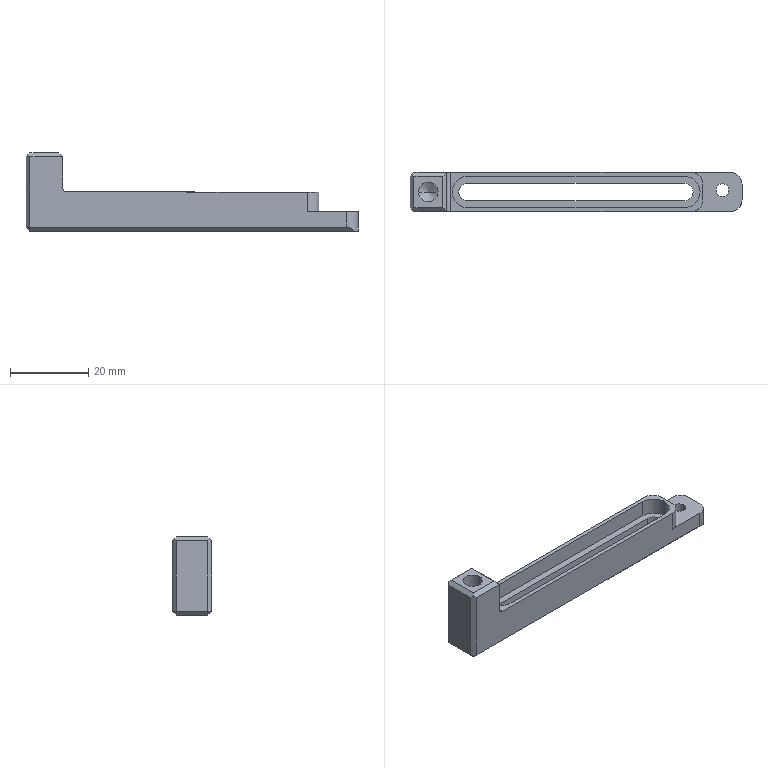Part | SolidWorks | features ICE 4, Chamfer 3, Fillet 3, HoleWzd 2, Extrusion 1 | 1 solid | 43 faces | box 85 x 10 x 20 mm | volume 4731 mm3 | plane 26 | cylinder 15 | cone 2 | commonest cylinder face diameters 6 x4 4.5 x3 8 x3 3.3 x2 5 x2 2 x1
STEP:
#1=CARTESIAN_POINT('',(35.85,5.5,-5.));
#2=VERTEX_POINT('',#1);
#3=CARTESIAN_POINT('',(39.15,5.5,-5.));
#4=VERTEX_POINT('',#3);
#5=CARTESIAN_POINT('',(37.5,5.5,-5.));
#6=DIRECTION('',(0.,0.,1.));
#7=DIRECTION('',(1.,0.,0.));
#8=AXIS2_PLACEMENT_3D('',#5,#6,#7);
#9=CIRCLE('',#8,1.65);
#10=EDGE_CURVE('',#2,#4,#9,.T.);
#11=ORIENTED_EDGE('',*,*,#10,.F.);
#12=CARTESIAN_POINT('',(35.85,5.5,0.));
#13=VERTEX_POINT('',#12);
#14=CARTESIAN_POINT('',(35.85,5.5,0.));
#15=DIRECTION('',(0.,0.,1.));
#16=VECTOR('',#15,1000.);
#17=LINE('',#14,#16);
#18=EDGE_CURVE('',#2,#13,#17,.T.);
#19=ORIENTED_EDGE('',*,*,#18,.T.);
#20=CARTESIAN_POINT('',(39.15,5.5,0.));
#21=VERTEX_POINT('',#20);
#22=CARTESIAN_POINT('',(37.5,5.5,0.));
#23=DIRECTION('',(0.,0.,1.));
#24=DIRECTION('',(1.,0.,0.));
#25=AXIS2_PLACEMENT_3D('',#22,#23,#24);
#26=CIRCLE('',#25,1.65);
#27=EDGE_CURVE('',#13,#21,#26,.T.);
#28=ORIENTED_EDGE('',*,*,#27,.T.);
#29=CARTESIAN_POINT('',(39.15,5.5,0.));
#30=DIRECTION('',(0.,0.,1.));
#31=VECTOR('',#30,1000.);
#32=LINE('',#29,#31);
#33=EDGE_CURVE('',#4,#21,#32,.T.);
#34=ORIENTED_EDGE('',*,*,#33,.F.);
#35=EDGE_LOOP('',(#11,#19,#28,#34));
#36=FACE_OUTER_BOUND('',#35,.T.);
#37=CARTESIAN_POINT('',(37.5,5.5,0.));
#38=DIRECTION('',(0.,0.,1.));
#39=DIRECTION('',(1.,0.,0.));
#40=AXIS2_PLACEMENT_3D('',#37,#38,#39);
#41=CYLINDRICAL_SURFACE('',#40,1.65);
#42=ADVANCED_FACE('',(#36),#41,.F.);
#43=CARTESIAN_POINT('',(-40.3,5.,-2.));
#44=VERTEX_POINT('',#43);
#45=CARTESIAN_POINT('',(-35.3,5.,-2.));
#46=VERTEX_POINT('',#45);
#47=CARTESIAN_POINT('',(-37.8,5.,-2.));
#48=DIRECTION('',(0.,0.,1.));
#49=DIRECTION('',(1.,0.,0.));
#50=AXIS2_PLACEMENT_3D('',#47,#48,#49);
#51=CIRCLE('',#50,2.5);
#52=EDGE_CURVE('',#44,#46,#51,.T.);
#53=ORIENTED_EDGE('',*,*,#52,.F.);
#54=CARTESIAN_POINT('',(-40.3,5.,15.));
#55=VERTEX_POINT('',#54);
#56=CARTESIAN_POINT('',(-40.3,5.,15.));
#57=DIRECTION('',(0.,0.,1.));
#58=VECTOR('',#57,1000.);
#59=LINE('',#56,#58);
#60=EDGE_CURVE('',#44,#55,#59,.T.);
#61=ORIENTED_EDGE('',*,*,#60,.T.);
#62=CARTESIAN_POINT('',(-35.3,5.,15.));
#63=VERTEX_POINT('',#62);
#64=CARTESIAN_POINT('',(-37.8,5.,15.));
#65=DIRECTION('',(0.,0.,1.));
#66=DIRECTION('',(1.,0.,0.));
#67=AXIS2_PLACEMENT_3D('',#64,#65,#66);
#68=CIRCLE('',#67,2.5);
#69=EDGE_CURVE('',#55,#63,#68,.T.);
#70=ORIENTED_EDGE('',*,*,#69,.T.);
#71=CARTESIAN_POINT('',(-35.3,5.,15.));
#72=DIRECTION('',(0.,0.,1.));
#73=VECTOR('',#72,1000.);
#74=LINE('',#71,#73);
#75=EDGE_CURVE('',#46,#63,#74,.T.);
#76=ORIENTED_EDGE('',*,*,#75,.F.);
#77=EDGE_LOOP('',(#53,#61,#70,#76));
#78=FACE_OUTER_BOUND('',#77,.T.);
#79=CARTESIAN_POINT('',(-37.8,5.,15.));
#80=DIRECTION('',(0.,0.,1.));
#81=DIRECTION('',(1.,0.,0.));
#82=AXIS2_PLACEMENT_3D('',#79,#80,#81);
#83=CYLINDRICAL_SURFACE('',#82,2.5);
#84=ADVANCED_FACE('',(#78),#83,.F.);
#85=CARTESIAN_POINT('',(-37.8,5.,-3.502));
#86=VERTEX_POINT('',#85);
#87=CARTESIAN_POINT('',(-35.3,5.,-2.));
#88=DIRECTION('',(0.8572,0.,0.515));
#89=VECTOR('',#88,1000.);
#90=LINE('',#87,#89);
#91=EDGE_CURVE('',#86,#46,#90,.T.);
#92=ORIENTED_EDGE('',*,*,#91,.F.);
#93=CARTESIAN_POINT('',(-40.3,5.,-2.));
#94=DIRECTION('',(-0.8572,0.,0.515));
#95=VECTOR('',#94,1000.);
#96=LINE('',#93,#95);
#97=EDGE_CURVE('',#86,#44,#96,.T.);
#98=ORIENTED_EDGE('',*,*,#97,.T.);
#99=ORIENTED_EDGE('',*,*,#52,.T.);
#100=EDGE_LOOP('',(#92,#98,#99));
#101=FACE_OUTER_BOUND('',#100,.T.);
#102=CARTESIAN_POINT('',(-37.8,5.,-2.));
#103=DIRECTION('',(0.,0.,1.));
#104=DIRECTION('',(1.,0.,0.));
#105=AXIS2_PLACEMENT_3D('',#102,#103,#104);
#106=CONICAL_SURFACE('',#105,2.5,1.03);
#107=ADVANCED_FACE('',(#101),#106,.F.);
#108=CARTESIAN_POINT('',(30.,5.,-5.));
#109=VERTEX_POINT('',#108);
#110=CARTESIAN_POINT('',(27.75,7.25,-5.));
#111=VERTEX_POINT('',#110);
#112=CARTESIAN_POINT('',(27.75,5.,-5.));
#113=DIRECTION('',(0.,0.,1.));
#114=DIRECTION('',(1.,0.,0.));
#115=AXIS2_PLACEMENT_3D('',#112,#113,#114);
#116=CIRCLE('',#115,2.25);
#117=EDGE_CURVE('',#109,#111,#116,.T.);
#118=ORIENTED_EDGE('',*,*,#117,.F.);
#119=CARTESIAN_POINT('',(30.,5.,0.6));
#120=VERTEX_POINT('',#119);
#121=CARTESIAN_POINT('',(30.,5.,-5.));
#122=DIRECTION('',(0.,0.,1.));
#123=VECTOR('',#122,1000.);
#124=LINE('',#121,#123);
#125=EDGE_CURVE('',#109,#120,#124,.T.);
#126=ORIENTED_EDGE('',*,*,#125,.T.);
#127=CARTESIAN_POINT('',(27.75,7.25,0.6));
#128=VERTEX_POINT('',#127);
#129=CARTESIAN_POINT('',(27.75,5.,0.6));
#130=DIRECTION('',(0.,0.,1.));
#131=DIRECTION('',(1.,0.,0.));
#132=AXIS2_PLACEMENT_3D('',#129,#130,#131);
#133=CIRCLE('',#132,2.25);
#134=EDGE_CURVE('',#120,#128,#133,.T.);
#135=ORIENTED_EDGE('',*,*,#134,.T.);
#136=CARTESIAN_POINT('',(27.75,7.25,-5.));
#137=DIRECTION('',(0.,0.,1.));
#138=VECTOR('',#137,1000.);
#139=LINE('',#136,#138);
#140=EDGE_CURVE('',#111,#128,#139,.T.);
#141=ORIENTED_EDGE('',*,*,#140,.F.);
#142=EDGE_LOOP('',(#118,#126,#135,#141));
#143=FACE_OUTER_BOUND('',#142,.T.);
#144=CARTESIAN_POINT('',(27.75,5.,-5.));
#145=DIRECTION('',(0.,0.,1.));
#146=DIRECTION('',(1.,0.,0.));
#147=AXIS2_PLACEMENT_3D('',#144,#145,#146);
#148=CYLINDRICAL_SURFACE('',#147,2.25);
#149=ADVANCED_FACE('',(#143),#148,.F.);
#150=CARTESIAN_POINT('',(31.75,5.,0.6));
#151=VERTEX_POINT('',#150);
#152=CARTESIAN_POINT('',(27.75,9.,0.6));
#153=VERTEX_POINT('',#152);
#154=CARTESIAN_POINT('',(27.75,5.,0.6));
#155=DIRECTION('',(0.,0.,1.));
#156=DIRECTION('',(1.,0.,0.));
#157=AXIS2_PLACEMENT_3D('',#154,#155,#156);
#158=CIRCLE('',#157,4.);
#159=EDGE_CURVE('',#151,#153,#158,.T.);
#160=ORIENTED_EDGE('',*,*,#159,.F.);
#161=CARTESIAN_POINT('',(31.75,5.,5.));
#162=VERTEX_POINT('',#161);
#163=CARTESIAN_POINT('',(31.75,5.,0.6));
#164=DIRECTION('',(0.,0.,1.));
#165=VECTOR('',#164,1000.);
#166=LINE('',#163,#165);
#167=EDGE_CURVE('',#151,#162,#166,.T.);
#168=ORIENTED_EDGE('',*,*,#167,.T.);
#169=CARTESIAN_POINT('',(27.75,9.,5.));
#170=VERTEX_POINT('',#169);
#171=CARTESIAN_POINT('',(27.75,5.,5.));
#172=DIRECTION('',(0.,0.,1.));
#173=DIRECTION('',(1.,0.,0.));
#174=AXIS2_PLACEMENT_3D('',#171,#172,#173);
#175=CIRCLE('',#174,4.);
#176=EDGE_CURVE('',#162,#170,#175,.T.);
#177=ORIENTED_EDGE('',*,*,#176,.T.);
#178=CARTESIAN_POINT('',(27.75,9.,0.6));
#179=DIRECTION('',(0.,0.,1.));
#180=VECTOR('',#179,1000.);
#181=LINE('',#178,#180);
#182=EDGE_CURVE('',#153,#170,#181,.T.);
#183=ORIENTED_EDGE('',*,*,#182,.F.);
#184=EDGE_LOOP('',(#160,#168,#177,#183));
#185=FACE_OUTER_BOUND('',#184,.T.);
#186=CARTESIAN_POINT('',(27.75,5.,0.6));
#187=DIRECTION('',(0.,0.,1.));
#188=DIRECTION('',(1.,0.,0.));
#189=AXIS2_PLACEMENT_3D('',#186,#187,#188);
#190=CYLINDRICAL_SURFACE('',#189,4.);
#191=ADVANCED_FACE('',(#185),#190,.F.);
#192=CARTESIAN_POINT('',(-42.5,1.,14.));
#193=VERTEX_POINT('',#192);
#194=CARTESIAN_POINT('',(-42.5,9.,14.));
#195=VERTEX_POINT('',#194);
#196=CARTESIAN_POINT('',(-42.5,10.,14.));
#197=DIRECTION('',(0.,1.,0.));
#198=VECTOR('',#197,1000.);
#199=LINE('',#196,#198);
#200=EDGE_CURVE('',#193,#195,#199,.T.);
#201=ORIENTED_EDGE('',*,*,#200,.T.);
#202=CARTESIAN_POINT('',(-42.5,9.,-4.));
#203=VERTEX_POINT('',#202);
#204=CARTESIAN_POINT('',(-42.5,9.,-5.));
#205=DIRECTION('',(0.,0.,-1.));
#206=VECTOR('',#205,1000.);
#207=LINE('',#204,#206);
#208=EDGE_CURVE('',#195,#203,#207,.T.);
#209=ORIENTED_EDGE('',*,*,#208,.T.);
#210=CARTESIAN_POINT('',(-42.5,1.,-4.));
#211=VERTEX_POINT('',#210);
#212=CARTESIAN_POINT('',(-42.5,10.,-4.));
#213=DIRECTION('',(0.,-1.,0.));
#214=VECTOR('',#213,1000.);
#215=LINE('',#212,#214);
#216=EDGE_CURVE('',#203,#211,#215,.T.);
#217=ORIENTED_EDGE('',*,*,#216,.T.);
#218=CARTESIAN_POINT('',(-42.5,1.,5.));
#219=DIRECTION('',(0.,0.,1.));
#220=VECTOR('',#219,1000.);
#221=LINE('',#218,#220);
#222=EDGE_CURVE('',#211,#193,#221,.T.);
#223=ORIENTED_EDGE('',*,*,#222,.T.);
#224=EDGE_LOOP('',(#201,#209,#217,#223));
#225=FACE_OUTER_BOUND('',#224,.T.);
#226=CARTESIAN_POINT('',(-42.5,10.,5.));
#227=DIRECTION('',(1.,0.,0.));
#228=DIRECTION('',(0.,0.,-1.));
#229=AXIS2_PLACEMENT_3D('',#226,#227,#228);
#230=PLANE('',#229);
#231=ADVANCED_FACE('',(#225),#230,.F.);
#232=CARTESIAN_POINT('',(-27.75,1.,5.));
#233=VERTEX_POINT('',#232);
#234=CARTESIAN_POINT('',(27.75,1.,5.));
#235=VERTEX_POINT('',#234);
#236=CARTESIAN_POINT('',(-27.75,1.,5.));
#237=DIRECTION('',(1.,0.,0.));
#238=VECTOR('',#237,1000.);
#239=LINE('',#236,#238);
#240=EDGE_CURVE('',#233,#235,#239,.T.);
#241=ORIENTED_EDGE('',*,*,#240,.F.);
#242=CARTESIAN_POINT('',(-27.75,9.,5.));
#243=VERTEX_POINT('',#242);
#244=CARTESIAN_POINT('',(-27.75,5.,5.));
#245=DIRECTION('',(0.,0.,1.));
#246=DIRECTION('',(1.,0.,0.));
#247=AXIS2_PLACEMENT_3D('',#244,#245,#246);
#248=CIRCLE('',#247,4.);
#249=EDGE_CURVE('',#243,#233,#248,.T.);
#250=ORIENTED_EDGE('',*,*,#249,.F.);
#251=CARTESIAN_POINT('',(-27.75,9.,5.));
#252=DIRECTION('',(-1.,0.,0.));
#253=VECTOR('',#252,1000.);
#254=LINE('',#251,#253);
#255=EDGE_CURVE('',#170,#243,#254,.T.);
#256=ORIENTED_EDGE('',*,*,#255,.F.);
#257=ORIENTED_EDGE('',*,*,#176,.F.);
#258=CARTESIAN_POINT('',(27.75,5.,5.));
#259=DIRECTION('',(0.,0.,1.));
#260=DIRECTION('',(1.,0.,0.));
#261=AXIS2_PLACEMENT_3D('',#258,#259,#260);
#262=CIRCLE('',#261,4.);
#263=EDGE_CURVE('',#235,#162,#262,.T.);
#264=ORIENTED_EDGE('',*,*,#263,.F.);
#265=EDGE_LOOP('',(#241,#250,#256,#257,#264));
#266=FACE_BOUND('',#265,.T.);
#267=CARTESIAN_POINT('',(-32.1,10.,5.));
#268=VERTEX_POINT('',#267);
#269=CARTESIAN_POINT('',(29.5,10.,5.));
#270=VERTEX_POINT('',#269);
#271=CARTESIAN_POINT('',(42.5,10.,5.));
#272=DIRECTION('',(1.,0.,0.));
#273=VECTOR('',#272,1000.);
#274=LINE('',#271,#273);
#275=EDGE_CURVE('',#268,#270,#274,.T.);
#276=ORIENTED_EDGE('',*,*,#275,.F.);
#277=CARTESIAN_POINT('',(-32.1,0.,5.));
#278=VERTEX_POINT('',#277);
#279=CARTESIAN_POINT('',(-32.1,10.,5.));
#280=DIRECTION('',(0.,-1.,0.));
#281=VECTOR('',#280,1000.);
#282=LINE('',#279,#281);
#283=EDGE_CURVE('',#268,#278,#282,.T.);
#284=ORIENTED_EDGE('',*,*,#283,.T.);
#285=CARTESIAN_POINT('',(29.5,0.,5.));
#286=VERTEX_POINT('',#285);
#287=CARTESIAN_POINT('',(42.5,0.,5.));
#288=DIRECTION('',(1.,0.,0.));
#289=VECTOR('',#288,1000.);
#290=LINE('',#287,#289);
#291=EDGE_CURVE('',#278,#286,#290,.T.);
#292=ORIENTED_EDGE('',*,*,#291,.T.);
#293=CARTESIAN_POINT('',(32.5,3.,5.));
#294=VERTEX_POINT('',#293);
#295=CARTESIAN_POINT('',(29.5,3.,5.));
#296=DIRECTION('',(0.,0.,1.));
#297=DIRECTION('',(-1.,0.,0.));
#298=AXIS2_PLACEMENT_3D('',#295,#296,#297);
#299=CIRCLE('',#298,3.);
#300=EDGE_CURVE('',#286,#294,#299,.T.);
#301=ORIENTED_EDGE('',*,*,#300,.T.);
#302=CARTESIAN_POINT('',(32.5,7.,5.));
#303=VERTEX_POINT('',#302);
#304=CARTESIAN_POINT('',(32.5,10.,5.));
#305=DIRECTION('',(0.,-1.,0.));
#306=VECTOR('',#305,1000.);
#307=LINE('',#304,#306);
#308=EDGE_CURVE('',#303,#294,#307,.T.);
#309=ORIENTED_EDGE('',*,*,#308,.F.);
#310=CARTESIAN_POINT('',(29.5,7.,5.));
#311=DIRECTION('',(0.,0.,1.));
#312=DIRECTION('',(-1.,0.,0.));
#313=AXIS2_PLACEMENT_3D('',#310,#311,#312);
#314=CIRCLE('',#313,3.);
#315=EDGE_CURVE('',#303,#270,#314,.T.);
#316=ORIENTED_EDGE('',*,*,#315,.T.);
#317=EDGE_LOOP('',(#276,#284,#292,#301,#309,#316));
#318=FACE_OUTER_BOUND('',#317,.T.);
#319=CARTESIAN_POINT('',(42.5,10.,5.));
#320=DIRECTION('',(0.,0.,-1.));
#321=DIRECTION('',(-1.,0.,0.));
#322=AXIS2_PLACEMENT_3D('',#319,#320,#321);
#323=PLANE('',#322);
#324=ADVANCED_FACE('',(#266,#318),#323,.F.);
#325=CARTESIAN_POINT('',(42.5,3.,0.));
#326=VERTEX_POINT('',#325);
#327=CARTESIAN_POINT('',(42.5,7.,0.));
#328=VERTEX_POINT('',#327);
#329=CARTESIAN_POINT('',(42.5,10.,0.));
#330=DIRECTION('',(0.,1.,0.));
#331=VECTOR('',#330,1000.);
#332=LINE('',#329,#331);
#333=EDGE_CURVE('',#326,#328,#332,.T.);
#334=ORIENTED_EDGE('',*,*,#333,.F.);
#335=CARTESIAN_POINT('',(42.5,3.,-5.));
#336=VERTEX_POINT('',#335);
#337=CARTESIAN_POINT('',(42.5,3.,5.));
#338=DIRECTION('',(0.,0.,-1.));
#339=VECTOR('',#338,1000.);
#340=LINE('',#337,#339);
#341=EDGE_CURVE('',#326,#336,#340,.T.);
#342=ORIENTED_EDGE('',*,*,#341,.T.);
#343=CARTESIAN_POINT('',(42.5,7.,-5.));
#344=VERTEX_POINT('',#343);
#345=CARTESIAN_POINT('',(42.5,10.,-5.));
#346=DIRECTION('',(0.,-1.,0.));
#347=VECTOR('',#346,1000.);
#348=LINE('',#345,#347);
#349=EDGE_CURVE('',#344,#336,#348,.T.);
#350=ORIENTED_EDGE('',*,*,#349,.F.);
#351=CARTESIAN_POINT('',(42.5,7.,0.));
#352=DIRECTION('',(0.,0.,1.));
#353=VECTOR('',#352,1000.);
#354=LINE('',#351,#353);
#355=EDGE_CURVE('',#344,#328,#354,.T.);
#356=ORIENTED_EDGE('',*,*,#355,.T.);
#357=EDGE_LOOP('',(#334,#342,#350,#356));
#358=FACE_OUTER_BOUND('',#357,.T.);
#359=CARTESIAN_POINT('',(42.5,10.,5.));
#360=DIRECTION('',(-1.,0.,0.));
#361=DIRECTION('',(0.,0.,1.));
#362=AXIS2_PLACEMENT_3D('',#359,#360,#361);
#363=PLANE('',#362);
#364=ADVANCED_FACE('',(#358),#363,.F.);
#365=CARTESIAN_POINT('',(37.5,5.5,-5.));
#366=DIRECTION('',(0.,0.,1.));
#367=DIRECTION('',(1.,0.,0.));
#368=AXIS2_PLACEMENT_3D('',#365,#366,#367);
#369=CIRCLE('',#368,1.65);
#370=EDGE_CURVE('',#4,#2,#369,.T.);
#371=ORIENTED_EDGE('',*,*,#370,.T.);
#372=ORIENTED_EDGE('',*,*,#10,.T.);
#373=EDGE_LOOP('',(#371,#372));
#374=FACE_BOUND('',#373,.T.);
#375=CARTESIAN_POINT('',(-27.75,7.25,-5.));
#376=VERTEX_POINT('',#375);
#377=CARTESIAN_POINT('',(-27.75,7.25,-5.));
#378=DIRECTION('',(-1.,0.,0.));
#379=VECTOR('',#378,1000.);
#380=LINE('',#377,#379);
#381=EDGE_CURVE('',#111,#376,#380,.T.);
#382=ORIENTED_EDGE('',*,*,#381,.T.);
#383=CARTESIAN_POINT('',(-27.75,2.75,-5.));
#384=VERTEX_POINT('',#383);
#385=CARTESIAN_POINT('',(-27.75,5.,-5.));
#386=DIRECTION('',(0.,0.,1.));
#387=DIRECTION('',(1.,0.,0.));
#388=AXIS2_PLACEMENT_3D('',#385,#386,#387);
#389=CIRCLE('',#388,2.25);
#390=EDGE_CURVE('',#376,#384,#389,.T.);
#391=ORIENTED_EDGE('',*,*,#390,.T.);
#392=CARTESIAN_POINT('',(27.75,2.75,-5.));
#393=VERTEX_POINT('',#392);
#394=CARTESIAN_POINT('',(-27.75,2.75,-5.));
#395=DIRECTION('',(1.,0.,0.));
#396=VECTOR('',#395,1000.);
#397=LINE('',#394,#396);
#398=EDGE_CURVE('',#384,#393,#397,.T.);
#399=ORIENTED_EDGE('',*,*,#398,.T.);
#400=CARTESIAN_POINT('',(27.75,5.,-5.));
#401=DIRECTION('',(0.,0.,1.));
#402=DIRECTION('',(1.,0.,0.));
#403=AXIS2_PLACEMENT_3D('',#400,#401,#402);
#404=CIRCLE('',#403,2.25);
#405=EDGE_CURVE('',#393,#109,#404,.T.);
#406=ORIENTED_EDGE('',*,*,#405,.T.);
#407=ORIENTED_EDGE('',*,*,#117,.T.);
#408=EDGE_LOOP('',(#382,#391,#399,#406,#407));
#409=FACE_BOUND('',#408,.T.);
#410=ORIENTED_EDGE('',*,*,#349,.T.);
#411=CARTESIAN_POINT('',(41.736,1.,-5.));
#412=VERTEX_POINT('',#411);
#413=CARTESIAN_POINT('',(39.5,3.,-5.));
#414=DIRECTION('',(0.,0.,-1.));
#415=DIRECTION('',(1.,0.,0.));
#416=AXIS2_PLACEMENT_3D('',#413,#414,#415);
#417=CIRCLE('',#416,3.);
#418=EDGE_CURVE('',#336,#412,#417,.T.);
#419=ORIENTED_EDGE('',*,*,#418,.T.);
#420=CARTESIAN_POINT('',(-41.5,1.,-5.));
#421=VERTEX_POINT('',#420);
#422=CARTESIAN_POINT('',(42.5,1.,-5.));
#423=DIRECTION('',(-1.,0.,0.));
#424=VECTOR('',#423,1000.);
#425=LINE('',#422,#424);
#426=EDGE_CURVE('',#412,#421,#425,.T.);
#427=ORIENTED_EDGE('',*,*,#426,.T.);
#428=CARTESIAN_POINT('',(-41.5,9.,-5.));
#429=VERTEX_POINT('',#428);
#430=CARTESIAN_POINT('',(-41.5,10.,-5.));
#431=DIRECTION('',(0.,1.,0.));
#432=VECTOR('',#431,1000.);
#433=LINE('',#430,#432);
#434=EDGE_CURVE('',#421,#429,#433,.T.);
#435=ORIENTED_EDGE('',*,*,#434,.T.);
#436=CARTESIAN_POINT('',(41.736,9.,-5.));
#437=VERTEX_POINT('',#436);
#438=CARTESIAN_POINT('',(42.5,9.,-5.));
#439=DIRECTION('',(1.,0.,0.));
#440=VECTOR('',#439,1000.);
#441=LINE('',#438,#440);
#442=EDGE_CURVE('',#429,#437,#441,.T.);
#443=ORIENTED_EDGE('',*,*,#442,.T.);
#444=CARTESIAN_POINT('',(39.5,7.,-5.));
#445=DIRECTION('',(0.,0.,-1.));
#446=DIRECTION('',(1.,0.,0.));
#447=AXIS2_PLACEMENT_3D('',#444,#445,#446);
#448=CIRCLE('',#447,3.);
#449=EDGE_CURVE('',#437,#344,#448,.T.);
#450=ORIENTED_EDGE('',*,*,#449,.T.);
#451=EDGE_LOOP('',(#410,#419,#427,#435,#443,#450));
#452=FACE_OUTER_BOUND('',#451,.T.);
#453=CARTESIAN_POINT('',(42.5,10.,-5.));
#454=DIRECTION('',(0.,0.,1.));
#455=DIRECTION('',(1.,0.,0.));
#456=AXIS2_PLACEMENT_3D('',#453,#454,#455);
#457=PLANE('',#456);
#458=ADVANCED_FACE('',(#374,#409,#452),#457,.F.);
#459=CARTESIAN_POINT('',(39.5,10.,0.));
#460=VERTEX_POINT('',#459);
#461=CARTESIAN_POINT('',(29.5,10.,0.));
#462=VERTEX_POINT('',#461);
#463=CARTESIAN_POINT('',(42.5,10.,0.));
#464=DIRECTION('',(-1.,0.,0.));
#465=VECTOR('',#464,1000.);
#466=LINE('',#463,#465);
#467=EDGE_CURVE('',#460,#462,#466,.T.);
#468=ORIENTED_EDGE('',*,*,#467,.F.);
#469=CARTESIAN_POINT('',(39.5,10.,-4.));
#470=VERTEX_POINT('',#469);
#471=CARTESIAN_POINT('',(39.5,10.,-4.));
#472=DIRECTION('',(0.,0.,-1.));
#473=VECTOR('',#472,1000.);
#474=LINE('',#471,#473);
#475=EDGE_CURVE('',#460,#470,#474,.T.);
#476=ORIENTED_EDGE('',*,*,#475,.T.);
#477=CARTESIAN_POINT('',(-41.5,10.,-4.));
#478=VERTEX_POINT('',#477);
#479=CARTESIAN_POINT('',(-42.5,10.,-4.));
#480=DIRECTION('',(-1.,0.,0.));
#481=VECTOR('',#480,1000.);
#482=LINE('',#479,#481);
#483=EDGE_CURVE('',#470,#478,#482,.T.);
#484=ORIENTED_EDGE('',*,*,#483,.T.);
#485=CARTESIAN_POINT('',(-41.5,10.,14.));
#486=VERTEX_POINT('',#485);
#487=CARTESIAN_POINT('',(-41.5,10.,14.));
#488=DIRECTION('',(0.,0.,1.));
#489=VECTOR('',#488,1000.);
#490=LINE('',#487,#489);
#491=EDGE_CURVE('',#478,#486,#490,.T.);
#492=ORIENTED_EDGE('',*,*,#491,.T.);
#493=CARTESIAN_POINT('',(-33.1,10.,14.));
#494=VERTEX_POINT('',#493);
#495=CARTESIAN_POINT('',(-33.1,10.,14.));
#496=DIRECTION('',(1.,0.,0.));
#497=VECTOR('',#496,1000.);
#498=LINE('',#495,#497);
#499=EDGE_CURVE('',#486,#494,#498,.T.);
#500=ORIENTED_EDGE('',*,*,#499,.T.);
#501=CARTESIAN_POINT('',(-33.1,10.,6.));
#502=VERTEX_POINT('',#501);
#503=CARTESIAN_POINT('',(-33.1,10.,15.));
#504=DIRECTION('',(0.,0.,-1.));
#505=VECTOR('',#504,1000.);
#506=LINE('',#503,#505);
#507=EDGE_CURVE('',#494,#502,#506,.T.);
#508=ORIENTED_EDGE('',*,*,#507,.T.);
#509=CARTESIAN_POINT('',(-32.1,10.,6.));
#510=DIRECTION('',(0.,-1.,0.));
#511=DIRECTION('',(0.,0.,1.));
#512=AXIS2_PLACEMENT_3D('',#509,#510,#511);
#513=CIRCLE('',#512,1.);
#514=EDGE_CURVE('',#502,#268,#513,.T.);
#515=ORIENTED_EDGE('',*,*,#514,.T.);
#516=ORIENTED_EDGE('',*,*,#275,.T.);
#517=CARTESIAN_POINT('',(29.5,10.,0.));
#518=DIRECTION('',(0.,0.,-1.));
#519=VECTOR('',#518,1000.);
#520=LINE('',#517,#519);
#521=EDGE_CURVE('',#270,#462,#520,.T.);
#522=ORIENTED_EDGE('',*,*,#521,.T.);
#523=EDGE_LOOP('',(#468,#476,#484,#492,#500,#508,#515,#516,#522));
#524=FACE_OUTER_BOUND('',#523,.T.);
#525=CARTESIAN_POINT('',(0.,10.,0.));
#526=DIRECTION('',(0.,1.,0.));
#527=DIRECTION('',(0.,0.,1.));
#528=AXIS2_PLACEMENT_3D('',#525,#526,#527);
#529=PLANE('',#528);
#530=ADVANCED_FACE('',(#524),#529,.T.);
#531=CARTESIAN_POINT('',(-41.5,0.,-4.));
#532=VERTEX_POINT('',#531);
#533=CARTESIAN_POINT('',(39.5,0.,-4.));
#534=VERTEX_POINT('',#533);
#535=CARTESIAN_POINT('',(0.,0.,-4.));
#536=DIRECTION('',(1.,0.,0.));
#537=VECTOR('',#536,1000.);
#538=LINE('',#535,#537);
#539=EDGE_CURVE('',#532,#534,#538,.T.);
#540=ORIENTED_EDGE('',*,*,#539,.T.);
#541=CARTESIAN_POINT('',(39.5,0.,0.));
#542=VERTEX_POINT('',#541);
#543=CARTESIAN_POINT('',(39.5,0.,0.));
#544=DIRECTION('',(0.,0.,1.));
#545=VECTOR('',#544,1000.);
#546=LINE('',#543,#545);
#547=EDGE_CURVE('',#534,#542,#546,.T.);
#548=ORIENTED_EDGE('',*,*,#547,.T.);
#549=CARTESIAN_POINT('',(29.5,0.,0.));
#550=VERTEX_POINT('',#549);
#551=CARTESIAN_POINT('',(42.5,0.,0.));
#552=DIRECTION('',(1.,0.,0.));
#553=VECTOR('',#552,1000.);
#554=LINE('',#551,#553);
#555=EDGE_CURVE('',#550,#542,#554,.T.);
#556=ORIENTED_EDGE('',*,*,#555,.F.);
#557=CARTESIAN_POINT('',(29.5,0.,0.));
#558=DIRECTION('',(0.,0.,1.));
#559=VECTOR('',#558,1000.);
#560=LINE('',#557,#559);
#561=EDGE_CURVE('',#550,#286,#560,.T.);
#562=ORIENTED_EDGE('',*,*,#561,.T.);
#563=ORIENTED_EDGE('',*,*,#291,.F.);
#564=CARTESIAN_POINT('',(-33.1,0.,6.));
#565=VERTEX_POINT('',#564);
#566=CARTESIAN_POINT('',(-32.1,0.,6.));
#567=DIRECTION('',(0.,1.,0.));
#568=DIRECTION('',(0.,0.,1.));
#569=AXIS2_PLACEMENT_3D('',#566,#567,#568);
#570=CIRCLE('',#569,1.);
#571=EDGE_CURVE('',#278,#565,#570,.T.);
#572=ORIENTED_EDGE('',*,*,#571,.T.);
#573=CARTESIAN_POINT('',(-33.1,0.,14.));
#574=VERTEX_POINT('',#573);
#575=CARTESIAN_POINT('',(-33.1,0.,15.));
#576=DIRECTION('',(0.,0.,-1.));
#577=VECTOR('',#576,1000.);
#578=LINE('',#575,#577);
#579=EDGE_CURVE('',#574,#565,#578,.T.);
#580=ORIENTED_EDGE('',*,*,#579,.F.);
#581=CARTESIAN_POINT('',(-41.5,0.,14.));
#582=VERTEX_POINT('',#581);
#583=CARTESIAN_POINT('',(0.,0.,14.));
#584=DIRECTION('',(-1.,0.,0.));
#585=VECTOR('',#584,1000.);
#586=LINE('',#583,#585);
#587=EDGE_CURVE('',#574,#582,#586,.T.);
#588=ORIENTED_EDGE('',*,*,#587,.T.);
#589=CARTESIAN_POINT('',(-41.5,0.,0.));
#590=DIRECTION('',(0.,0.,-1.));
#591=VECTOR('',#590,1000.);
#592=LINE('',#589,#591);
#593=EDGE_CURVE('',#582,#532,#592,.T.);
#594=ORIENTED_EDGE('',*,*,#593,.T.);
#595=EDGE_LOOP('',(#540,#548,#556,#562,#563,#572,#580,#588,#594));
#596=FACE_OUTER_BOUND('',#595,.T.);
#597=CARTESIAN_POINT('',(0.,0.,0.));
#598=DIRECTION('',(0.,1.,0.));
#599=DIRECTION('',(0.,0.,1.));
#600=AXIS2_PLACEMENT_3D('',#597,#598,#599);
#601=PLANE('',#600);
#602=ADVANCED_FACE('',(#596),#601,.F.);
#603=ORIENTED_EDGE('',*,*,#249,.T.);
#604=CARTESIAN_POINT('',(-27.75,1.,0.6));
#605=VERTEX_POINT('',#604);
#606=CARTESIAN_POINT('',(-27.75,1.,0.6));
#607=DIRECTION('',(0.,0.,1.));
#608=VECTOR('',#607,1000.);
#609=LINE('',#606,#608);
#610=EDGE_CURVE('',#605,#233,#609,.T.);
#611=ORIENTED_EDGE('',*,*,#610,.F.);
#612=CARTESIAN_POINT('',(-27.75,9.,0.6));
#613=VERTEX_POINT('',#612);
#614=CARTESIAN_POINT('',(-27.75,5.,0.6));
#615=DIRECTION('',(0.,0.,1.));
#616=DIRECTION('',(1.,0.,0.));
#617=AXIS2_PLACEMENT_3D('',#614,#615,#616);
#618=CIRCLE('',#617,4.);
#619=EDGE_CURVE('',#613,#605,#618,.T.);
#620=ORIENTED_EDGE('',*,*,#619,.F.);
#621=CARTESIAN_POINT('',(-27.75,9.,0.6));
#622=DIRECTION('',(0.,0.,1.));
#623=VECTOR('',#622,1000.);
#624=LINE('',#621,#623);
#625=EDGE_CURVE('',#613,#243,#624,.T.);
#626=ORIENTED_EDGE('',*,*,#625,.T.);
#627=EDGE_LOOP('',(#603,#611,#620,#626));
#628=FACE_OUTER_BOUND('',#627,.T.);
#629=CARTESIAN_POINT('',(-27.75,5.,0.6));
#630=DIRECTION('',(0.,0.,1.));
#631=DIRECTION('',(1.,0.,0.));
#632=AXIS2_PLACEMENT_3D('',#629,#630,#631);
#633=CYLINDRICAL_SURFACE('',#632,4.);
#634=ADVANCED_FACE('',(#628),#633,.F.);
#635=ORIENTED_EDGE('',*,*,#255,.T.);
#636=ORIENTED_EDGE('',*,*,#625,.F.);
#637=CARTESIAN_POINT('',(-27.75,9.,0.6));
#638=DIRECTION('',(-1.,0.,0.));
#639=VECTOR('',#638,1000.);
#640=LINE('',#637,#639);
#641=EDGE_CURVE('',#153,#613,#640,.T.);
#642=ORIENTED_EDGE('',*,*,#641,.F.);
#643=ORIENTED_EDGE('',*,*,#182,.T.);
#644=EDGE_LOOP('',(#635,#636,#642,#643));
#645=FACE_OUTER_BOUND('',#644,.T.);
#646=CARTESIAN_POINT('',(-27.75,9.,0.6));
#647=DIRECTION('',(0.,1.,0.));
#648=DIRECTION('',(-1.,0.,0.));
#649=AXIS2_PLACEMENT_3D('',#646,#647,#648);
#650=PLANE('',#649);
#651=ADVANCED_FACE('',(#645),#650,.F.);
#652=ORIENTED_EDGE('',*,*,#167,.F.);
#653=CARTESIAN_POINT('',(27.75,1.,0.6));
#654=VERTEX_POINT('',#653);
#655=CARTESIAN_POINT('',(27.75,5.,0.6));
#656=DIRECTION('',(0.,0.,1.));
#657=DIRECTION('',(1.,0.,0.));
#658=AXIS2_PLACEMENT_3D('',#655,#656,#657);
#659=CIRCLE('',#658,4.);
#660=EDGE_CURVE('',#654,#151,#659,.T.);
#661=ORIENTED_EDGE('',*,*,#660,.F.);
#662=CARTESIAN_POINT('',(27.75,1.,0.6));
#663=DIRECTION('',(0.,0.,1.));
#664=VECTOR('',#663,1000.);
#665=LINE('',#662,#664);
#666=EDGE_CURVE('',#654,#235,#665,.T.);
#667=ORIENTED_EDGE('',*,*,#666,.T.);
#668=ORIENTED_EDGE('',*,*,#263,.T.);
#669=EDGE_LOOP('',(#652,#661,#667,#668));
#670=FACE_OUTER_BOUND('',#669,.T.);
#671=CARTESIAN_POINT('',(27.75,5.,0.6));
#672=DIRECTION('',(0.,0.,1.));
#673=DIRECTION('',(1.,0.,0.));
#674=AXIS2_PLACEMENT_3D('',#671,#672,#673);
#675=CYLINDRICAL_SURFACE('',#674,4.);
#676=ADVANCED_FACE('',(#670),#675,.F.);
#677=ORIENTED_EDGE('',*,*,#240,.T.);
#678=ORIENTED_EDGE('',*,*,#666,.F.);
#679=CARTESIAN_POINT('',(-27.75,1.,0.6));
#680=DIRECTION('',(1.,0.,0.));
#681=VECTOR('',#680,1000.);
#682=LINE('',#679,#681);
#683=EDGE_CURVE('',#605,#654,#682,.T.);
#684=ORIENTED_EDGE('',*,*,#683,.F.);
#685=ORIENTED_EDGE('',*,*,#610,.T.);
#686=EDGE_LOOP('',(#677,#678,#684,#685));
#687=FACE_OUTER_BOUND('',#686,.T.);
#688=CARTESIAN_POINT('',(-27.75,1.,0.6));
#689=DIRECTION('',(0.,-1.,0.));
#690=DIRECTION('',(1.,0.,0.));
#691=AXIS2_PLACEMENT_3D('',#688,#689,#690);
#692=PLANE('',#691);
#693=ADVANCED_FACE('',(#687),#692,.F.);
#694=CARTESIAN_POINT('',(-27.75,7.25,0.6));
#695=VERTEX_POINT('',#694);
#696=CARTESIAN_POINT('',(-27.75,2.75,0.6));
#697=VERTEX_POINT('',#696);
#698=CARTESIAN_POINT('',(-27.75,5.,0.6));
#699=DIRECTION('',(0.,0.,1.));
#700=DIRECTION('',(1.,0.,0.));
#701=AXIS2_PLACEMENT_3D('',#698,#699,#700);
#702=CIRCLE('',#701,2.25);
#703=EDGE_CURVE('',#695,#697,#702,.T.);
#704=ORIENTED_EDGE('',*,*,#703,.F.);
#705=CARTESIAN_POINT('',(-27.75,7.25,0.6));
#706=DIRECTION('',(-1.,0.,0.));
#707=VECTOR('',#706,1000.);
#708=LINE('',#705,#707);
#709=EDGE_CURVE('',#128,#695,#708,.T.);
#710=ORIENTED_EDGE('',*,*,#709,.F.);
#711=ORIENTED_EDGE('',*,*,#134,.F.);
#712=CARTESIAN_POINT('',(27.75,2.75,0.6));
#713=VERTEX_POINT('',#712);
#714=CARTESIAN_POINT('',(27.75,5.,0.6));
#715=DIRECTION('',(0.,0.,1.));
#716=DIRECTION('',(1.,0.,0.));
#717=AXIS2_PLACEMENT_3D('',#714,#715,#716);
#718=CIRCLE('',#717,2.25);
#719=EDGE_CURVE('',#713,#120,#718,.T.);
#720=ORIENTED_EDGE('',*,*,#719,.F.);
#721=CARTESIAN_POINT('',(-27.75,2.75,0.6));
#722=DIRECTION('',(1.,0.,0.));
#723=VECTOR('',#722,1000.);
#724=LINE('',#721,#723);
#725=EDGE_CURVE('',#697,#713,#724,.T.);
#726=ORIENTED_EDGE('',*,*,#725,.F.);
#727=EDGE_LOOP('',(#704,#710,#711,#720,#726));
#728=FACE_BOUND('',#727,.T.);
#729=ORIENTED_EDGE('',*,*,#619,.T.);
#730=ORIENTED_EDGE('',*,*,#683,.T.);
#731=ORIENTED_EDGE('',*,*,#660,.T.);
#732=ORIENTED_EDGE('',*,*,#159,.T.);
#733=ORIENTED_EDGE('',*,*,#641,.T.);
#734=EDGE_LOOP('',(#729,#730,#731,#732,#733));
#735=FACE_OUTER_BOUND('',#734,.T.);
#736=CARTESIAN_POINT('',(-27.75,5.,0.6));
#737=DIRECTION('',(0.,0.,1.));
#738=DIRECTION('',(1.,0.,0.));
#739=AXIS2_PLACEMENT_3D('',#736,#737,#738);
#740=PLANE('',#739);
#741=ADVANCED_FACE('',(#728,#735),#740,.T.);
#742=ORIENTED_EDGE('',*,*,#703,.T.);
#743=CARTESIAN_POINT('',(-27.75,2.75,-5.));
#744=DIRECTION('',(0.,0.,1.));
#745=VECTOR('',#744,1000.);
#746=LINE('',#743,#745);
#747=EDGE_CURVE('',#384,#697,#746,.T.);
#748=ORIENTED_EDGE('',*,*,#747,.F.);
#749=ORIENTED_EDGE('',*,*,#390,.F.);
#750=CARTESIAN_POINT('',(-27.75,7.25,-5.));
#751=DIRECTION('',(0.,0.,1.));
#752=VECTOR('',#751,1000.);
#753=LINE('',#750,#752);
#754=EDGE_CURVE('',#376,#695,#753,.T.);
#755=ORIENTED_EDGE('',*,*,#754,.T.);
#756=EDGE_LOOP('',(#742,#748,#749,#755));
#757=FACE_OUTER_BOUND('',#756,.T.);
#758=CARTESIAN_POINT('',(-27.75,5.,-5.));
#759=DIRECTION('',(0.,0.,1.));
#760=DIRECTION('',(1.,0.,0.));
#761=AXIS2_PLACEMENT_3D('',#758,#759,#760);
#762=CYLINDRICAL_SURFACE('',#761,2.25);
#763=ADVANCED_FACE('',(#757),#762,.F.);
#764=ORIENTED_EDGE('',*,*,#709,.T.);
#765=ORIENTED_EDGE('',*,*,#754,.F.);
#766=ORIENTED_EDGE('',*,*,#381,.F.);
#767=ORIENTED_EDGE('',*,*,#140,.T.);
#768=EDGE_LOOP('',(#764,#765,#766,#767));
#769=FACE_OUTER_BOUND('',#768,.T.);
#770=CARTESIAN_POINT('',(-27.75,7.25,-5.));
#771=DIRECTION('',(0.,1.,0.));
#772=DIRECTION('',(0.,0.,1.));
#773=AXIS2_PLACEMENT_3D('',#770,#771,#772);
#774=PLANE('',#773);
#775=ADVANCED_FACE('',(#769),#774,.F.);
#776=ORIENTED_EDGE('',*,*,#125,.F.);
#777=ORIENTED_EDGE('',*,*,#405,.F.);
#778=CARTESIAN_POINT('',(27.75,2.75,-5.));
#779=DIRECTION('',(0.,0.,1.));
#780=VECTOR('',#779,1000.);
#781=LINE('',#778,#780);
#782=EDGE_CURVE('',#393,#713,#781,.T.);
#783=ORIENTED_EDGE('',*,*,#782,.T.);
#784=ORIENTED_EDGE('',*,*,#719,.T.);
#785=EDGE_LOOP('',(#776,#777,#783,#784));
#786=FACE_OUTER_BOUND('',#785,.T.);
#787=CARTESIAN_POINT('',(27.75,5.,-5.));
#788=DIRECTION('',(0.,0.,1.));
#789=DIRECTION('',(1.,0.,0.));
#790=AXIS2_PLACEMENT_3D('',#787,#788,#789);
#791=CYLINDRICAL_SURFACE('',#790,2.25);
#792=ADVANCED_FACE('',(#786),#791,.F.);
#793=ORIENTED_EDGE('',*,*,#725,.T.);
#794=ORIENTED_EDGE('',*,*,#782,.F.);
#795=ORIENTED_EDGE('',*,*,#398,.F.);
#796=ORIENTED_EDGE('',*,*,#747,.T.);
#797=EDGE_LOOP('',(#793,#794,#795,#796));
#798=FACE_OUTER_BOUND('',#797,.T.);
#799=CARTESIAN_POINT('',(-27.75,2.75,-5.));
#800=DIRECTION('',(0.,-1.,0.));
#801=DIRECTION('',(0.,0.,-1.));
#802=AXIS2_PLACEMENT_3D('',#799,#800,#801);
#803=PLANE('',#802);
#804=ADVANCED_FACE('',(#798),#803,.F.);
#805=ORIENTED_EDGE('',*,*,#579,.T.);
#806=CARTESIAN_POINT('',(-33.1,10.,6.));
#807=DIRECTION('',(0.,1.,0.));
#808=VECTOR('',#807,1000.);
#809=LINE('',#806,#808);
#810=EDGE_CURVE('',#565,#502,#809,.T.);
#811=ORIENTED_EDGE('',*,*,#810,.T.);
#812=ORIENTED_EDGE('',*,*,#507,.F.);
#813=CARTESIAN_POINT('',(-33.1,0.,14.));
#814=DIRECTION('',(0.,-1.,0.));
#815=VECTOR('',#814,1000.);
#816=LINE('',#813,#815);
#817=EDGE_CURVE('',#494,#574,#816,.T.);
#818=ORIENTED_EDGE('',*,*,#817,.T.);
#819=EDGE_LOOP('',(#805,#811,#812,#818));
#820=FACE_OUTER_BOUND('',#819,.T.);
#821=CARTESIAN_POINT('',(-33.1,10.,15.));
#822=DIRECTION('',(1.,0.,0.));
#823=DIRECTION('',(0.,0.,-1.));
#824=AXIS2_PLACEMENT_3D('',#821,#822,#823);
#825=PLANE('',#824);
#826=ADVANCED_FACE('',(#820),#825,.T.);
#827=CARTESIAN_POINT('',(-34.1,9.,15.));
#828=VERTEX_POINT('',#827);
#829=CARTESIAN_POINT('',(-41.5,9.,15.));
#830=VERTEX_POINT('',#829);
#831=CARTESIAN_POINT('',(-42.5,9.,15.));
#832=DIRECTION('',(-1.,0.,0.));
#833=VECTOR('',#832,1000.);
#834=LINE('',#831,#833);
#835=EDGE_CURVE('',#828,#830,#834,.T.);
#836=ORIENTED_EDGE('',*,*,#835,.T.);
#837=CARTESIAN_POINT('',(-41.5,1.,15.));
#838=VERTEX_POINT('',#837);
#839=CARTESIAN_POINT('',(-41.5,0.,15.));
#840=DIRECTION('',(0.,-1.,0.));
#841=VECTOR('',#840,1000.);
#842=LINE('',#839,#841);
#843=EDGE_CURVE('',#830,#838,#842,.T.);
#844=ORIENTED_EDGE('',*,*,#843,.T.);
#845=CARTESIAN_POINT('',(-34.1,1.,15.));
#846=VERTEX_POINT('',#845);
#847=CARTESIAN_POINT('',(0.,1.,15.));
#848=DIRECTION('',(1.,0.,0.));
#849=VECTOR('',#848,1000.);
#850=LINE('',#847,#849);
#851=EDGE_CURVE('',#838,#846,#850,.T.);
#852=ORIENTED_EDGE('',*,*,#851,.T.);
#853=CARTESIAN_POINT('',(-34.1,10.,15.));
#854=DIRECTION('',(0.,1.,0.));
#855=VECTOR('',#854,1000.);
#856=LINE('',#853,#855);
#857=EDGE_CURVE('',#846,#828,#856,.T.);
#858=ORIENTED_EDGE('',*,*,#857,.T.);
#859=EDGE_LOOP('',(#836,#844,#852,#858));
#860=FACE_OUTER_BOUND('',#859,.T.);
#861=CARTESIAN_POINT('',(-37.8,5.,15.));
#862=DIRECTION('',(0.,0.,1.));
#863=DIRECTION('',(1.,0.,0.));
#864=AXIS2_PLACEMENT_3D('',#861,#862,#863);
#865=CIRCLE('',#864,2.5);
#866=EDGE_CURVE('',#63,#55,#865,.T.);
#867=ORIENTED_EDGE('',*,*,#866,.F.);
#868=ORIENTED_EDGE('',*,*,#69,.F.);
#869=EDGE_LOOP('',(#867,#868));
#870=FACE_BOUND('',#869,.T.);
#871=CARTESIAN_POINT('',(0.,0.,15.));
#872=DIRECTION('',(0.,0.,-1.));
#873=DIRECTION('',(-1.,0.,0.));
#874=AXIS2_PLACEMENT_3D('',#871,#872,#873);
#875=PLANE('',#874);
#876=ADVANCED_FACE('',(#860,#870),#875,.F.);
#877=ORIENTED_EDGE('',*,*,#308,.T.);
#878=CARTESIAN_POINT('',(32.5,3.,0.));
#879=VERTEX_POINT('',#878);
#880=CARTESIAN_POINT('',(32.5,3.,0.));
#881=DIRECTION('',(0.,0.,-1.));
#882=VECTOR('',#881,1000.);
#883=LINE('',#880,#882);
#884=EDGE_CURVE('',#294,#879,#883,.T.);
#885=ORIENTED_EDGE('',*,*,#884,.T.);
#886=CARTESIAN_POINT('',(32.5,7.,0.));
#887=VERTEX_POINT('',#886);
#888=CARTESIAN_POINT('',(32.5,10.,0.));
#889=DIRECTION('',(0.,-1.,0.));
#890=VECTOR('',#889,1000.);
#891=LINE('',#888,#890);
#892=EDGE_CURVE('',#887,#879,#891,.T.);
#893=ORIENTED_EDGE('',*,*,#892,.F.);
#894=CARTESIAN_POINT('',(32.5,7.,5.));
#895=DIRECTION('',(0.,0.,1.));
#896=VECTOR('',#895,1000.);
#897=LINE('',#894,#896);
#898=EDGE_CURVE('',#887,#303,#897,.T.);
#899=ORIENTED_EDGE('',*,*,#898,.T.);
#900=EDGE_LOOP('',(#877,#885,#893,#899));
#901=FACE_OUTER_BOUND('',#900,.T.);
#902=CARTESIAN_POINT('',(32.5,10.,0.));
#903=DIRECTION('',(-1.,0.,0.));
#904=DIRECTION('',(0.,0.,1.));
#905=AXIS2_PLACEMENT_3D('',#902,#903,#904);
#906=PLANE('',#905);
#907=ADVANCED_FACE('',(#901),#906,.F.);
#908=CARTESIAN_POINT('',(37.5,5.5,0.));
#909=DIRECTION('',(0.,0.,1.));
#910=DIRECTION('',(1.,0.,0.));
#911=AXIS2_PLACEMENT_3D('',#908,#909,#910);
#912=CIRCLE('',#911,1.65);
#913=EDGE_CURVE('',#21,#13,#912,.T.);
#914=ORIENTED_EDGE('',*,*,#913,.F.);
#915=ORIENTED_EDGE('',*,*,#27,.F.);
#916=EDGE_LOOP('',(#914,#915));
#917=FACE_BOUND('',#916,.T.);
#918=ORIENTED_EDGE('',*,*,#555,.T.);
#919=CARTESIAN_POINT('',(39.5,3.,0.));
#920=DIRECTION('',(0.,0.,1.));
#921=DIRECTION('',(-1.,0.,0.));
#922=AXIS2_PLACEMENT_3D('',#919,#920,#921);
#923=CIRCLE('',#922,3.);
#924=EDGE_CURVE('',#542,#326,#923,.T.);
#925=ORIENTED_EDGE('',*,*,#924,.T.);
#926=ORIENTED_EDGE('',*,*,#333,.T.);
#927=CARTESIAN_POINT('',(39.5,7.,0.));
#928=DIRECTION('',(0.,0.,1.));
#929=DIRECTION('',(-1.,0.,0.));
#930=AXIS2_PLACEMENT_3D('',#927,#928,#929);
#931=CIRCLE('',#930,3.);
#932=EDGE_CURVE('',#328,#460,#931,.T.);
#933=ORIENTED_EDGE('',*,*,#932,.T.);
#934=ORIENTED_EDGE('',*,*,#467,.T.);
#935=CARTESIAN_POINT('',(29.5,7.,0.));
#936=DIRECTION('',(0.,0.,-1.));
#937=DIRECTION('',(-1.,0.,0.));
#938=AXIS2_PLACEMENT_3D('',#935,#936,#937);
#939=CIRCLE('',#938,3.);
#940=EDGE_CURVE('',#462,#887,#939,.T.);
#941=ORIENTED_EDGE('',*,*,#940,.T.);
#942=ORIENTED_EDGE('',*,*,#892,.T.);
#943=CARTESIAN_POINT('',(29.5,3.,0.));
#944=DIRECTION('',(0.,0.,-1.));
#945=DIRECTION('',(-1.,0.,0.));
#946=AXIS2_PLACEMENT_3D('',#943,#944,#945);
#947=CIRCLE('',#946,3.);
#948=EDGE_CURVE('',#879,#550,#947,.T.);
#949=ORIENTED_EDGE('',*,*,#948,.T.);
#950=EDGE_LOOP('',(#918,#925,#926,#933,#934,#941,#942,#949));
#951=FACE_OUTER_BOUND('',#950,.T.);
#952=CARTESIAN_POINT('',(0.,0.,0.));
#953=DIRECTION('',(0.,0.,-1.));
#954=DIRECTION('',(-1.,0.,0.));
#955=AXIS2_PLACEMENT_3D('',#952,#953,#954);
#956=PLANE('',#955);
#957=ADVANCED_FACE('',(#917,#951),#956,.F.);
#958=ORIENTED_EDGE('',*,*,#97,.F.);
#959=ORIENTED_EDGE('',*,*,#91,.T.);
#960=CARTESIAN_POINT('',(-37.8,5.,-2.));
#961=DIRECTION('',(0.,0.,1.));
#962=DIRECTION('',(1.,0.,0.));
#963=AXIS2_PLACEMENT_3D('',#960,#961,#962);
#964=CIRCLE('',#963,2.5);
#965=EDGE_CURVE('',#46,#44,#964,.T.);
#966=ORIENTED_EDGE('',*,*,#965,.T.);
#967=EDGE_LOOP('',(#958,#959,#966));
#968=FACE_OUTER_BOUND('',#967,.T.);
#969=CARTESIAN_POINT('',(-37.8,5.,-2.));
#970=DIRECTION('',(0.,0.,1.));
#971=DIRECTION('',(1.,0.,0.));
#972=AXIS2_PLACEMENT_3D('',#969,#970,#971);
#973=CONICAL_SURFACE('',#972,2.5,1.03);
#974=ADVANCED_FACE('',(#968),#973,.F.);
#975=ORIENTED_EDGE('',*,*,#60,.F.);
#976=ORIENTED_EDGE('',*,*,#965,.F.);
#977=ORIENTED_EDGE('',*,*,#75,.T.);
#978=ORIENTED_EDGE('',*,*,#866,.T.);
#979=EDGE_LOOP('',(#975,#976,#977,#978));
#980=FACE_OUTER_BOUND('',#979,.T.);
#981=CARTESIAN_POINT('',(-37.8,5.,15.));
#982=DIRECTION('',(0.,0.,1.));
#983=DIRECTION('',(1.,0.,0.));
#984=AXIS2_PLACEMENT_3D('',#981,#982,#983);
#985=CYLINDRICAL_SURFACE('',#984,2.5);
#986=ADVANCED_FACE('',(#980),#985,.F.);
#987=ORIENTED_EDGE('',*,*,#18,.F.);
#988=ORIENTED_EDGE('',*,*,#370,.F.);
#989=ORIENTED_EDGE('',*,*,#33,.T.);
#990=ORIENTED_EDGE('',*,*,#913,.T.);
#991=EDGE_LOOP('',(#987,#988,#989,#990));
#992=FACE_OUTER_BOUND('',#991,.T.);
#993=CARTESIAN_POINT('',(37.5,5.5,0.));
#994=DIRECTION('',(0.,0.,1.));
#995=DIRECTION('',(1.,0.,0.));
#996=AXIS2_PLACEMENT_3D('',#993,#994,#995);
#997=CYLINDRICAL_SURFACE('',#996,1.65);
#998=ADVANCED_FACE('',(#992),#997,.F.);
#999=ORIENTED_EDGE('',*,*,#948,.F.);
#1000=ORIENTED_EDGE('',*,*,#884,.F.);
#1001=ORIENTED_EDGE('',*,*,#300,.F.);
#1002=ORIENTED_EDGE('',*,*,#561,.F.);
#1003=EDGE_LOOP('',(#999,#1000,#1001,#1002));
#1004=FACE_OUTER_BOUND('',#1003,.T.);
#1005=CARTESIAN_POINT('',(29.5,3.,0.));
#1006=DIRECTION('',(0.,0.,1.));
#1007=DIRECTION('',(1.,0.,0.));
#1008=AXIS2_PLACEMENT_3D('',#1005,#1006,#1007);
#1009=CYLINDRICAL_SURFACE('',#1008,3.);
#1010=ADVANCED_FACE('',(#1004),#1009,.T.);
#1011=ORIENTED_EDGE('',*,*,#940,.F.);
#1012=ORIENTED_EDGE('',*,*,#521,.F.);
#1013=ORIENTED_EDGE('',*,*,#315,.F.);
#1014=ORIENTED_EDGE('',*,*,#898,.F.);
#1015=EDGE_LOOP('',(#1011,#1012,#1013,#1014));
#1016=FACE_OUTER_BOUND('',#1015,.T.);
#1017=CARTESIAN_POINT('',(29.5,7.,0.));
#1018=DIRECTION('',(0.,0.,-1.));
#1019=DIRECTION('',(-1.,0.,0.));
#1020=AXIS2_PLACEMENT_3D('',#1017,#1018,#1019);
#1021=CYLINDRICAL_SURFACE('',#1020,3.);
#1022=ADVANCED_FACE('',(#1016),#1021,.T.);
#1023=CARTESIAN_POINT('',(-22.733,-10.367,3.633));
#1024=DIRECTION('',(-0.5774,0.5774,0.5774));
#1025=VECTOR('',#1024,1000.);
#1026=LINE('',#1023,#1025);
#1027=EDGE_CURVE('',#574,#846,#1026,.T.);
#1028=ORIENTED_EDGE('',*,*,#1027,.F.);
#1029=ORIENTED_EDGE('',*,*,#817,.F.);
#1030=CARTESIAN_POINT('',(-33.1,10.,14.));
#1031=DIRECTION('',(0.5774,0.5774,-0.5774));
#1032=VECTOR('',#1031,1000.);
#1033=LINE('',#1030,#1032);
#1034=EDGE_CURVE('',#828,#494,#1033,.T.);
#1035=ORIENTED_EDGE('',*,*,#1034,.F.);
#1036=ORIENTED_EDGE('',*,*,#857,.F.);
#1037=EDGE_LOOP('',(#1028,#1029,#1035,#1036));
#1038=FACE_OUTER_BOUND('',#1037,.T.);
#1039=CARTESIAN_POINT('',(-33.1,10.,14.));
#1040=DIRECTION('',(0.7071,0.,0.7071));
#1041=DIRECTION('',(0.,1.,0.));
#1042=AXIS2_PLACEMENT_3D('',#1039,#1040,#1041);
#1043=PLANE('',#1042);
#1044=ADVANCED_FACE('',(#1038),#1043,.T.);
#1045=ORIENTED_EDGE('',*,*,#499,.F.);
#1046=CARTESIAN_POINT('',(-42.,9.5,14.5));
#1047=VERTEX_POINT('',#1046);
#1048=CARTESIAN_POINT('',(-27.667,23.833,0.1667));
#1049=DIRECTION('',(-0.5774,-0.5774,0.5774));
#1050=VECTOR('',#1049,1000.);
#1051=LINE('',#1048,#1050);
#1052=EDGE_CURVE('',#486,#1047,#1051,.T.);
#1053=ORIENTED_EDGE('',*,*,#1052,.T.);
#1054=CARTESIAN_POINT('',(-28.333,-4.167,28.167));
#1055=DIRECTION('',(-0.5774,0.5774,-0.5774));
#1056=VECTOR('',#1055,1000.);
#1057=LINE('',#1054,#1056);
#1058=EDGE_CURVE('',#830,#1047,#1057,.T.);
#1059=ORIENTED_EDGE('',*,*,#1058,.F.);
#1060=ORIENTED_EDGE('',*,*,#835,.F.);
#1061=ORIENTED_EDGE('',*,*,#1034,.T.);
#1062=EDGE_LOOP('',(#1045,#1053,#1059,#1060,#1061));
#1063=FACE_OUTER_BOUND('',#1062,.T.);
#1064=CARTESIAN_POINT('',(0.,10.,14.));
#1065=DIRECTION('',(0.,0.7071,0.7071));
#1066=DIRECTION('',(-1.,0.,0.));
#1067=AXIS2_PLACEMENT_3D('',#1064,#1065,#1066);
#1068=PLANE('',#1067);
#1069=ADVANCED_FACE('',(#1063),#1068,.T.);
#1070=CARTESIAN_POINT('',(-42.,0.5,14.5));
#1071=VERTEX_POINT('',#1070);
#1072=CARTESIAN_POINT('',(-27.667,14.833,28.833));
#1073=DIRECTION('',(0.5774,0.5774,0.5774));
#1074=VECTOR('',#1073,1000.);
#1075=LINE('',#1072,#1074);
#1076=EDGE_CURVE('',#1071,#838,#1075,.T.);
#1077=ORIENTED_EDGE('',*,*,#1076,.F.);
#1078=CARTESIAN_POINT('',(-28.333,-13.167,0.8333));
#1079=DIRECTION('',(0.5774,-0.5774,-0.5774));
#1080=VECTOR('',#1079,1000.);
#1081=LINE('',#1078,#1080);
#1082=EDGE_CURVE('',#1071,#582,#1081,.T.);
#1083=ORIENTED_EDGE('',*,*,#1082,.T.);
#1084=ORIENTED_EDGE('',*,*,#587,.F.);
#1085=ORIENTED_EDGE('',*,*,#1027,.T.);
#1086=ORIENTED_EDGE('',*,*,#851,.F.);
#1087=EDGE_LOOP('',(#1077,#1083,#1084,#1085,#1086));
#1088=FACE_OUTER_BOUND('',#1087,.T.);
#1089=CARTESIAN_POINT('',(0.,1.,15.));
#1090=DIRECTION('',(0.,0.7071,-0.7071));
#1091=DIRECTION('',(1.,0.,0.));
#1092=AXIS2_PLACEMENT_3D('',#1089,#1090,#1091);
#1093=PLANE('',#1092);
#1094=ADVANCED_FACE('',(#1088),#1093,.F.);
#1095=ORIENTED_EDGE('',*,*,#1058,.T.);
#1096=CARTESIAN_POINT('',(-44.833,6.667,11.667));
#1097=DIRECTION('',(-0.5774,-0.5774,-0.5774));
#1098=VECTOR('',#1097,1000.);
#1099=LINE('',#1096,#1098);
#1100=EDGE_CURVE('',#1047,#195,#1099,.T.);
#1101=ORIENTED_EDGE('',*,*,#1100,.T.);
#1102=ORIENTED_EDGE('',*,*,#200,.F.);
#1103=CARTESIAN_POINT('',(-41.5,0.,15.));
#1104=DIRECTION('',(0.5774,-0.5774,0.5774));
#1105=VECTOR('',#1104,1000.);
#1106=LINE('',#1103,#1105);
#1107=EDGE_CURVE('',#193,#1071,#1106,.T.);
#1108=ORIENTED_EDGE('',*,*,#1107,.T.);
#1109=ORIENTED_EDGE('',*,*,#1076,.T.);
#1110=ORIENTED_EDGE('',*,*,#843,.F.);
#1111=EDGE_LOOP('',(#1095,#1101,#1102,#1108,#1109,#1110));
#1112=FACE_OUTER_BOUND('',#1111,.T.);
#1113=CARTESIAN_POINT('',(-41.5,0.,15.));
#1114=DIRECTION('',(0.7071,0.,-0.7071));
#1115=DIRECTION('',(0.,-1.,0.));
#1116=AXIS2_PLACEMENT_3D('',#1113,#1114,#1115);
#1117=PLANE('',#1116);
#1118=ADVANCED_FACE('',(#1112),#1117,.F.);
#1119=ORIENTED_EDGE('',*,*,#514,.F.);
#1120=ORIENTED_EDGE('',*,*,#810,.F.);
#1121=ORIENTED_EDGE('',*,*,#571,.F.);
#1122=ORIENTED_EDGE('',*,*,#283,.F.);
#1123=EDGE_LOOP('',(#1119,#1120,#1121,#1122));
#1124=FACE_OUTER_BOUND('',#1123,.T.);
#1125=CARTESIAN_POINT('',(-32.1,10.,6.));
#1126=DIRECTION('',(0.,-1.,0.));
#1127=DIRECTION('',(0.,0.,-1.));
#1128=AXIS2_PLACEMENT_3D('',#1125,#1126,#1127);
#1129=CYLINDRICAL_SURFACE('',#1128,1.);
#1130=ADVANCED_FACE('',(#1124),#1129,.F.);
#1131=ORIENTED_EDGE('',*,*,#1107,.F.);
#1132=ORIENTED_EDGE('',*,*,#222,.F.);
#1133=CARTESIAN_POINT('',(-42.,0.5,-4.));
#1134=DIRECTION('',(-0.7071,0.7071,0.));
#1135=VECTOR('',#1134,1000.);
#1136=LINE('',#1133,#1135);
#1137=EDGE_CURVE('',#532,#211,#1136,.T.);
#1138=ORIENTED_EDGE('',*,*,#1137,.F.);
#1139=ORIENTED_EDGE('',*,*,#593,.F.);
#1140=ORIENTED_EDGE('',*,*,#1082,.F.);
#1141=EDGE_LOOP('',(#1131,#1132,#1138,#1139,#1140));
#1142=FACE_OUTER_BOUND('',#1141,.T.);
#1143=CARTESIAN_POINT('',(-42.5,1.,5.));
#1144=DIRECTION('',(0.7071,0.7071,0.));
#1145=DIRECTION('',(0.,0.,1.));
#1146=AXIS2_PLACEMENT_3D('',#1143,#1144,#1145);
#1147=PLANE('',#1146);
#1148=ADVANCED_FACE('',(#1142),#1147,.F.);
#1149=ORIENTED_EDGE('',*,*,#426,.F.);
#1150=CARTESIAN_POINT('',(41.736,1.,-5.));
#1151=CARTESIAN_POINT('',(41.158,0.3539,-4.354));
#1152=CARTESIAN_POINT('',(40.367,0.,-4.));
#1153=CARTESIAN_POINT('',(39.5,0.,-4.));
#1154=(BOUNDED_CURVE()B_SPLINE_CURVE(3,(#1150,#1151,#1152,#1153),.UNSPECIFIED.,.F.,.F.)B_SPLINE_CURVE_WITH_KNOTS((4,4),(2.301,3.142),.UNSPECIFIED.)CURVE()GEOMETRIC_REPRESENTATION_ITEM()RATIONAL_B_SPLINE_CURVE((1.,0.9419,0.9419,1.))REPRESENTATION_ITEM(''));
#1155=EDGE_CURVE('',#412,#534,#1154,.T.);
#1156=ORIENTED_EDGE('',*,*,#1155,.T.);
#1157=ORIENTED_EDGE('',*,*,#539,.F.);
#1158=CARTESIAN_POINT('',(-41.5,1.,-5.));
#1159=DIRECTION('',(0.,-0.7071,0.7071));
#1160=VECTOR('',#1159,1000.);
#1161=LINE('',#1158,#1160);
#1162=EDGE_CURVE('',#421,#532,#1161,.T.);
#1163=ORIENTED_EDGE('',*,*,#1162,.F.);
#1164=EDGE_LOOP('',(#1149,#1156,#1157,#1163));
#1165=FACE_OUTER_BOUND('',#1164,.T.);
#1166=CARTESIAN_POINT('',(42.5,1.,-5.));
#1167=DIRECTION('',(0.,0.7071,0.7071));
#1168=DIRECTION('',(-1.,0.,0.));
#1169=AXIS2_PLACEMENT_3D('',#1166,#1167,#1168);
#1170=PLANE('',#1169);
#1171=ADVANCED_FACE('',(#1165),#1170,.F.);
#1172=ORIENTED_EDGE('',*,*,#1162,.T.);
#1173=ORIENTED_EDGE('',*,*,#1137,.T.);
#1174=CARTESIAN_POINT('',(-41.5,1.,-5.));
#1175=DIRECTION('',(-0.7071,0.,0.7071));
#1176=VECTOR('',#1175,1000.);
#1177=LINE('',#1174,#1176);
#1178=EDGE_CURVE('',#421,#211,#1177,.T.);
#1179=ORIENTED_EDGE('',*,*,#1178,.F.);
#1180=EDGE_LOOP('',(#1172,#1173,#1179));
#1181=FACE_OUTER_BOUND('',#1180,.T.);
#1182=CARTESIAN_POINT('',(-41.5,1.,-5.));
#1183=DIRECTION('',(-0.5774,-0.5774,-0.5774));
#1184=DIRECTION('',(0.,0.7071,-0.7071));
#1185=AXIS2_PLACEMENT_3D('',#1182,#1183,#1184);
#1186=PLANE('',#1185);
#1187=ADVANCED_FACE('',(#1181),#1186,.T.);
#1188=ORIENTED_EDGE('',*,*,#1052,.F.);
#1189=ORIENTED_EDGE('',*,*,#491,.F.);
#1190=CARTESIAN_POINT('',(-41.5,10.,-4.));
#1191=DIRECTION('',(0.7071,0.7071,0.));
#1192=VECTOR('',#1191,1000.);
#1193=LINE('',#1190,#1192);
#1194=EDGE_CURVE('',#203,#478,#1193,.T.);
#1195=ORIENTED_EDGE('',*,*,#1194,.F.);
#1196=ORIENTED_EDGE('',*,*,#208,.F.);
#1197=ORIENTED_EDGE('',*,*,#1100,.F.);
#1198=EDGE_LOOP('',(#1188,#1189,#1195,#1196,#1197));
#1199=FACE_OUTER_BOUND('',#1198,.T.);
#1200=CARTESIAN_POINT('',(-41.5,10.,0.));
#1201=DIRECTION('',(-0.7071,0.7071,0.));
#1202=DIRECTION('',(0.,0.,-1.));
#1203=AXIS2_PLACEMENT_3D('',#1200,#1201,#1202);
#1204=PLANE('',#1203);
#1205=ADVANCED_FACE('',(#1199),#1204,.T.);
#1206=ORIENTED_EDGE('',*,*,#1178,.T.);
#1207=ORIENTED_EDGE('',*,*,#216,.F.);
#1208=CARTESIAN_POINT('',(-42.,9.,-4.5));
#1209=DIRECTION('',(-0.7071,0.,0.7071));
#1210=VECTOR('',#1209,1000.);
#1211=LINE('',#1208,#1210);
#1212=EDGE_CURVE('',#429,#203,#1211,.T.);
#1213=ORIENTED_EDGE('',*,*,#1212,.F.);
#1214=ORIENTED_EDGE('',*,*,#434,.F.);
#1215=EDGE_LOOP('',(#1206,#1207,#1213,#1214));
#1216=FACE_OUTER_BOUND('',#1215,.T.);
#1217=CARTESIAN_POINT('',(-42.5,10.,-4.));
#1218=DIRECTION('',(0.7071,0.,0.7071));
#1219=DIRECTION('',(0.,-1.,0.));
#1220=AXIS2_PLACEMENT_3D('',#1217,#1218,#1219);
#1221=PLANE('',#1220);
#1222=ADVANCED_FACE('',(#1216),#1221,.F.);
#1223=ORIENTED_EDGE('',*,*,#1212,.T.);
#1224=ORIENTED_EDGE('',*,*,#1194,.T.);
#1225=CARTESIAN_POINT('',(-41.5,10.,-4.));
#1226=DIRECTION('',(0.,0.7071,0.7071));
#1227=VECTOR('',#1226,1000.);
#1228=LINE('',#1225,#1227);
#1229=EDGE_CURVE('',#429,#478,#1228,.T.);
#1230=ORIENTED_EDGE('',*,*,#1229,.F.);
#1231=EDGE_LOOP('',(#1223,#1224,#1230));
#1232=FACE_OUTER_BOUND('',#1231,.T.);
#1233=CARTESIAN_POINT('',(-41.5,10.,-4.));
#1234=DIRECTION('',(-0.5774,0.5774,-0.5774));
#1235=DIRECTION('',(0.,0.7071,0.7071));
#1236=AXIS2_PLACEMENT_3D('',#1233,#1234,#1235);
#1237=PLANE('',#1236);
#1238=ADVANCED_FACE('',(#1232),#1237,.T.);
#1239=ORIENTED_EDGE('',*,*,#483,.F.);
#1240=CARTESIAN_POINT('',(39.5,10.,-4.));
#1241=CARTESIAN_POINT('',(40.367,10.,-4.));
#1242=CARTESIAN_POINT('',(41.158,9.646,-4.354));
#1243=CARTESIAN_POINT('',(41.736,9.,-5.));
#1244=(BOUNDED_CURVE()B_SPLINE_CURVE(3,(#1240,#1241,#1242,#1243),.UNSPECIFIED.,.F.,.F.)B_SPLINE_CURVE_WITH_KNOTS((4,4),(0.,0.8411),.UNSPECIFIED.)CURVE()GEOMETRIC_REPRESENTATION_ITEM()RATIONAL_B_SPLINE_CURVE((1.,0.9419,0.9419,1.))REPRESENTATION_ITEM(''));
#1245=EDGE_CURVE('',#470,#437,#1244,.T.);
#1246=ORIENTED_EDGE('',*,*,#1245,.T.);
#1247=ORIENTED_EDGE('',*,*,#442,.F.);
#1248=ORIENTED_EDGE('',*,*,#1229,.T.);
#1249=EDGE_LOOP('',(#1239,#1246,#1247,#1248));
#1250=FACE_OUTER_BOUND('',#1249,.T.);
#1251=CARTESIAN_POINT('',(0.,10.,-4.));
#1252=DIRECTION('',(0.,0.7071,-0.7071));
#1253=DIRECTION('',(1.,0.,0.));
#1254=AXIS2_PLACEMENT_3D('',#1251,#1252,#1253);
#1255=PLANE('',#1254);
#1256=ADVANCED_FACE('',(#1250),#1255,.T.);
#1257=ORIENTED_EDGE('',*,*,#924,.F.);
#1258=ORIENTED_EDGE('',*,*,#547,.F.);
#1259=ORIENTED_EDGE('',*,*,#1155,.F.);
#1260=ORIENTED_EDGE('',*,*,#418,.F.);
#1261=ORIENTED_EDGE('',*,*,#341,.F.);
#1262=EDGE_LOOP('',(#1257,#1258,#1259,#1260,#1261));
#1263=FACE_OUTER_BOUND('',#1262,.T.);
#1264=CARTESIAN_POINT('',(39.5,3.,5.));
#1265=DIRECTION('',(0.,0.,-1.));
#1266=DIRECTION('',(-1.,0.,0.));
#1267=AXIS2_PLACEMENT_3D('',#1264,#1265,#1266);
#1268=CYLINDRICAL_SURFACE('',#1267,3.);
#1269=ADVANCED_FACE('',(#1263),#1268,.T.);
#1270=ORIENTED_EDGE('',*,*,#932,.F.);
#1271=ORIENTED_EDGE('',*,*,#355,.F.);
#1272=ORIENTED_EDGE('',*,*,#449,.F.);
#1273=ORIENTED_EDGE('',*,*,#1245,.F.);
#1274=ORIENTED_EDGE('',*,*,#475,.F.);
#1275=EDGE_LOOP('',(#1270,#1271,#1272,#1273,#1274));
#1276=FACE_OUTER_BOUND('',#1275,.T.);
#1277=CARTESIAN_POINT('',(39.5,7.,0.));
#1278=DIRECTION('',(0.,0.,1.));
#1279=DIRECTION('',(1.,0.,0.));
#1280=AXIS2_PLACEMENT_3D('',#1277,#1278,#1279);
#1281=CYLINDRICAL_SURFACE('',#1280,3.);
#1282=ADVANCED_FACE('',(#1276),#1281,.T.);
#1283=CLOSED_SHELL('',(#42,#84,#107,#149,#191,#231,#324,#364,#458,#530,#602,#634,#651,#676,#693,#741,#763,#775,#792,#804,#826,#876,#907,#957,#974,#986,#998,#1010,#1022,#1044,#1069,#1094,#1118,#1130,#1148,#1171,#1187,#1205,#1222,#1238,#1256,#1269,#1282));
#1284=MANIFOLD_SOLID_BREP('',#1283);
#1285=CARTESIAN_POINT('',(0.,0.,0.));
#1286=DIRECTION('',(0.,0.,1.));
#1287=DIRECTION('',(1.,0.,0.));
#1288=AXIS2_PLACEMENT_3D('',#1285,#1286,#1287);
#1289=(LENGTH_UNIT()NAMED_UNIT(*)SI_UNIT(.MILLI.,.METRE.));
#1290=UNCERTAINTY_MEASURE_WITH_UNIT(LENGTH_MEASURE(0.00001),#1289,'','');
#1291=(NAMED_UNIT(*)PLANE_ANGLE_UNIT()SI_UNIT($,.RADIAN.));
#1292=(NAMED_UNIT(*)SI_UNIT($,.STERADIAN.)SOLID_ANGLE_UNIT());
#1293=(GEOMETRIC_REPRESENTATION_CONTEXT(3)GLOBAL_UNCERTAINTY_ASSIGNED_CONTEXT((#1290))GLOBAL_UNIT_ASSIGNED_CONTEXT((#1289,#1291,#1292))REPRESENTATION_CONTEXT('',''));
#1294=ADVANCED_BREP_SHAPE_REPRESENTATION('',(#1284,#1288),#1293);